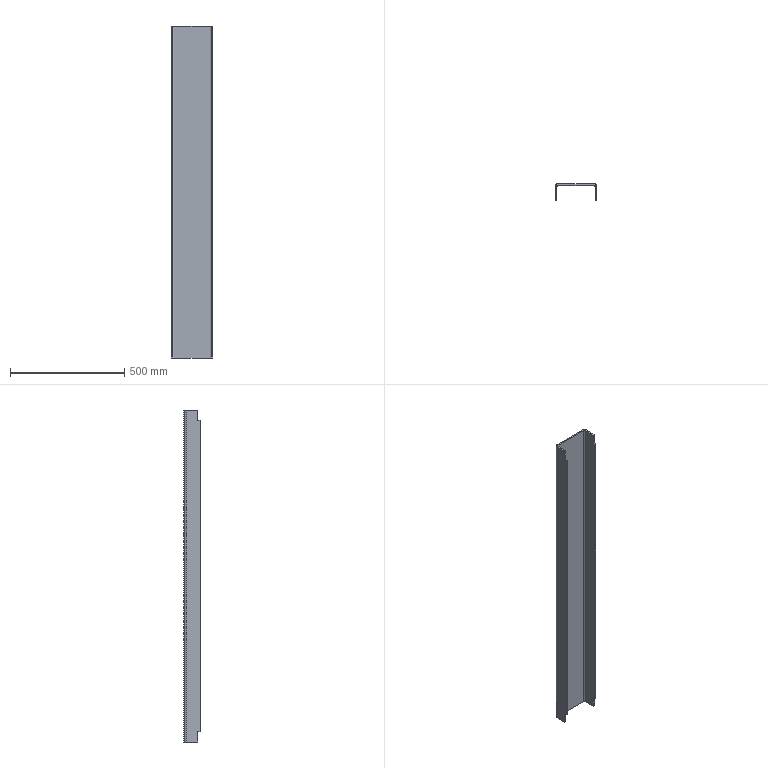Part | STEP file | VD-SYL0380DJ1006_1_1_2-1_VD-SYL | 1 solid | 30 faces | box 180 x 70 x 1450 mm | volume 2609055 mm3 | plane 26 | cylinder 4 | commonest cylinder face diameters 10 x2 22 x2
STEP:
#1=CARTESIAN_POINT('',(-90.,10.,725.));
#2=VERTEX_POINT('',#1);
#3=CARTESIAN_POINT('',(-90.,10.,680.));
#4=VERTEX_POINT('',#3);
#5=CARTESIAN_POINT('',(-90.,10.,725.));
#6=DIRECTION('',(0.,0.,-1.));
#7=VECTOR('',#6,1000.);
#8=LINE('',#5,#7);
#9=EDGE_CURVE('',#2,#4,#8,.T.);
#10=ORIENTED_EDGE('',*,*,#9,.F.);
#11=CARTESIAN_POINT('',(-90.,59.,725.));
#12=VERTEX_POINT('',#11);
#13=CARTESIAN_POINT('',(-90.,59.,725.));
#14=DIRECTION('',(0.,-1.,0.));
#15=VECTOR('',#14,1000.);
#16=LINE('',#13,#15);
#17=EDGE_CURVE('',#12,#2,#16,.T.);
#18=ORIENTED_EDGE('',*,*,#17,.F.);
#19=CARTESIAN_POINT('',(-90.,59.,-725.));
#20=VERTEX_POINT('',#19);
#21=CARTESIAN_POINT('',(-90.,59.,-725.));
#22=DIRECTION('',(0.,0.,1.));
#23=VECTOR('',#22,1000.);
#24=LINE('',#21,#23);
#25=EDGE_CURVE('',#20,#12,#24,.T.);
#26=ORIENTED_EDGE('',*,*,#25,.F.);
#27=CARTESIAN_POINT('',(-90.,10.,-725.));
#28=VERTEX_POINT('',#27);
#29=CARTESIAN_POINT('',(-90.,59.,-725.));
#30=DIRECTION('',(0.,-1.,0.));
#31=VECTOR('',#30,1000.);
#32=LINE('',#29,#31);
#33=EDGE_CURVE('',#20,#28,#32,.T.);
#34=ORIENTED_EDGE('',*,*,#33,.T.);
#35=CARTESIAN_POINT('',(-90.,10.,-680.));
#36=VERTEX_POINT('',#35);
#37=CARTESIAN_POINT('',(-90.,10.,-725.));
#38=DIRECTION('',(0.,0.,1.));
#39=VECTOR('',#38,1000.);
#40=LINE('',#37,#39);
#41=EDGE_CURVE('',#28,#36,#40,.T.);
#42=ORIENTED_EDGE('',*,*,#41,.T.);
#43=CARTESIAN_POINT('',(-90.,0.,-680.));
#44=VERTEX_POINT('',#43);
#45=CARTESIAN_POINT('',(-90.,0.,-680.));
#46=DIRECTION('',(0.,1.,0.));
#47=VECTOR('',#46,1000.);
#48=LINE('',#45,#47);
#49=EDGE_CURVE('',#44,#36,#48,.T.);
#50=ORIENTED_EDGE('',*,*,#49,.F.);
#51=CARTESIAN_POINT('',(-90.,0.,680.));
#52=VERTEX_POINT('',#51);
#53=CARTESIAN_POINT('',(-90.,0.,-680.));
#54=DIRECTION('',(0.,0.,1.));
#55=VECTOR('',#54,1000.);
#56=LINE('',#53,#55);
#57=EDGE_CURVE('',#44,#52,#56,.T.);
#58=ORIENTED_EDGE('',*,*,#57,.T.);
#59=CARTESIAN_POINT('',(-90.,0.,680.));
#60=DIRECTION('',(0.,1.,0.));
#61=VECTOR('',#60,1000.);
#62=LINE('',#59,#61);
#63=EDGE_CURVE('',#52,#4,#62,.T.);
#64=ORIENTED_EDGE('',*,*,#63,.T.);
#65=EDGE_LOOP('',(#10,#18,#26,#34,#42,#50,#58,#64));
#66=FACE_OUTER_BOUND('',#65,.T.);
#67=CARTESIAN_POINT('',(-90.,70.,-725.));
#68=DIRECTION('',(-1.,0.,0.));
#69=DIRECTION('',(0.,0.,1.));
#70=AXIS2_PLACEMENT_3D('',#67,#68,#69);
#71=PLANE('',#70);
#72=ADVANCED_FACE('',(#66),#71,.T.);
#73=ORIENTED_EDGE('',*,*,#25,.T.);
#74=CARTESIAN_POINT('',(-79.,70.,725.));
#75=VERTEX_POINT('',#74);
#76=CARTESIAN_POINT('',(-79.,59.,725.));
#77=DIRECTION('',(0.,0.,1.));
#78=DIRECTION('',(0.,1.,0.));
#79=AXIS2_PLACEMENT_3D('',#76,#77,#78);
#80=CIRCLE('',#79,11.);
#81=EDGE_CURVE('',#75,#12,#80,.T.);
#82=ORIENTED_EDGE('',*,*,#81,.F.);
#83=CARTESIAN_POINT('',(-79.,70.,-725.));
#84=VERTEX_POINT('',#83);
#85=CARTESIAN_POINT('',(-79.,70.,725.));
#86=DIRECTION('',(0.,0.,-1.));
#87=VECTOR('',#86,1000.);
#88=LINE('',#85,#87);
#89=EDGE_CURVE('',#75,#84,#88,.T.);
#90=ORIENTED_EDGE('',*,*,#89,.T.);
#91=CARTESIAN_POINT('',(-79.,59.,-725.));
#92=DIRECTION('',(0.,0.,-1.));
#93=DIRECTION('',(-1.,0.,0.));
#94=AXIS2_PLACEMENT_3D('',#91,#92,#93);
#95=CIRCLE('',#94,11.);
#96=EDGE_CURVE('',#20,#84,#95,.T.);
#97=ORIENTED_EDGE('',*,*,#96,.F.);
#98=EDGE_LOOP('',(#73,#82,#90,#97));
#99=FACE_OUTER_BOUND('',#98,.T.);
#100=CARTESIAN_POINT('',(-79.,59.,-725.));
#101=DIRECTION('',(0.,0.,-1.));
#102=DIRECTION('',(-1.,0.,0.));
#103=AXIS2_PLACEMENT_3D('',#100,#101,#102);
#104=CYLINDRICAL_SURFACE('',#103,11.);
#105=ADVANCED_FACE('',(#99),#104,.T.);
#106=CARTESIAN_POINT('',(79.,70.,-725.));
#107=VERTEX_POINT('',#106);
#108=CARTESIAN_POINT('',(79.,70.,-725.));
#109=DIRECTION('',(-1.,0.,0.));
#110=VECTOR('',#109,1000.);
#111=LINE('',#108,#110);
#112=EDGE_CURVE('',#107,#84,#111,.T.);
#113=ORIENTED_EDGE('',*,*,#112,.T.);
#114=ORIENTED_EDGE('',*,*,#89,.F.);
#115=CARTESIAN_POINT('',(79.,70.,725.));
#116=VERTEX_POINT('',#115);
#117=CARTESIAN_POINT('',(79.,70.,725.));
#118=DIRECTION('',(-1.,0.,0.));
#119=VECTOR('',#118,1000.);
#120=LINE('',#117,#119);
#121=EDGE_CURVE('',#116,#75,#120,.T.);
#122=ORIENTED_EDGE('',*,*,#121,.F.);
#123=CARTESIAN_POINT('',(79.,70.,-725.));
#124=DIRECTION('',(0.,0.,1.));
#125=VECTOR('',#124,1000.);
#126=LINE('',#123,#125);
#127=EDGE_CURVE('',#107,#116,#126,.T.);
#128=ORIENTED_EDGE('',*,*,#127,.F.);
#129=EDGE_LOOP('',(#113,#114,#122,#128));
#130=FACE_OUTER_BOUND('',#129,.T.);
#131=CARTESIAN_POINT('',(90.,70.,-725.));
#132=DIRECTION('',(0.,1.,0.));
#133=DIRECTION('',(1.,0.,0.));
#134=AXIS2_PLACEMENT_3D('',#131,#132,#133);
#135=PLANE('',#134);
#136=ADVANCED_FACE('',(#130),#135,.T.);
#137=ORIENTED_EDGE('',*,*,#127,.T.);
#138=CARTESIAN_POINT('',(90.,59.,725.));
#139=VERTEX_POINT('',#138);
#140=CARTESIAN_POINT('',(79.,59.,725.));
#141=DIRECTION('',(0.,0.,1.));
#142=DIRECTION('',(1.,0.,0.));
#143=AXIS2_PLACEMENT_3D('',#140,#141,#142);
#144=CIRCLE('',#143,11.);
#145=EDGE_CURVE('',#139,#116,#144,.T.);
#146=ORIENTED_EDGE('',*,*,#145,.F.);
#147=CARTESIAN_POINT('',(90.,59.,-725.));
#148=VERTEX_POINT('',#147);
#149=CARTESIAN_POINT('',(90.,59.,725.));
#150=DIRECTION('',(0.,0.,-1.));
#151=VECTOR('',#150,1000.);
#152=LINE('',#149,#151);
#153=EDGE_CURVE('',#139,#148,#152,.T.);
#154=ORIENTED_EDGE('',*,*,#153,.T.);
#155=CARTESIAN_POINT('',(79.,59.,-725.));
#156=DIRECTION('',(0.,0.,-1.));
#157=DIRECTION('',(0.,1.,0.));
#158=AXIS2_PLACEMENT_3D('',#155,#156,#157);
#159=CIRCLE('',#158,11.);
#160=EDGE_CURVE('',#107,#148,#159,.T.);
#161=ORIENTED_EDGE('',*,*,#160,.F.);
#162=EDGE_LOOP('',(#137,#146,#154,#161));
#163=FACE_OUTER_BOUND('',#162,.T.);
#164=CARTESIAN_POINT('',(79.,59.,-725.));
#165=DIRECTION('',(0.,0.,-1.));
#166=DIRECTION('',(-1.,0.,0.));
#167=AXIS2_PLACEMENT_3D('',#164,#165,#166);
#168=CYLINDRICAL_SURFACE('',#167,11.);
#169=ADVANCED_FACE('',(#163),#168,.T.);
#170=CARTESIAN_POINT('',(79.,64.,725.));
#171=VERTEX_POINT('',#170);
#172=CARTESIAN_POINT('',(-79.,64.,725.));
#173=VERTEX_POINT('',#172);
#174=CARTESIAN_POINT('',(79.,64.,725.));
#175=DIRECTION('',(-1.,0.,0.));
#176=VECTOR('',#175,1000.);
#177=LINE('',#174,#176);
#178=EDGE_CURVE('',#171,#173,#177,.T.);
#179=ORIENTED_EDGE('',*,*,#178,.T.);
#180=CARTESIAN_POINT('',(-79.,64.,-725.));
#181=VERTEX_POINT('',#180);
#182=CARTESIAN_POINT('',(-79.,64.,-725.));
#183=DIRECTION('',(0.,0.,1.));
#184=VECTOR('',#183,1000.);
#185=LINE('',#182,#184);
#186=EDGE_CURVE('',#181,#173,#185,.T.);
#187=ORIENTED_EDGE('',*,*,#186,.F.);
#188=CARTESIAN_POINT('',(79.,64.,-725.));
#189=VERTEX_POINT('',#188);
#190=CARTESIAN_POINT('',(79.,64.,-725.));
#191=DIRECTION('',(-1.,0.,0.));
#192=VECTOR('',#191,1000.);
#193=LINE('',#190,#192);
#194=EDGE_CURVE('',#189,#181,#193,.T.);
#195=ORIENTED_EDGE('',*,*,#194,.F.);
#196=CARTESIAN_POINT('',(79.,64.,725.));
#197=DIRECTION('',(0.,0.,-1.));
#198=VECTOR('',#197,1000.);
#199=LINE('',#196,#198);
#200=EDGE_CURVE('',#171,#189,#199,.T.);
#201=ORIENTED_EDGE('',*,*,#200,.F.);
#202=EDGE_LOOP('',(#179,#187,#195,#201));
#203=FACE_OUTER_BOUND('',#202,.T.);
#204=CARTESIAN_POINT('',(90.,64.,-725.));
#205=DIRECTION('',(0.,1.,0.));
#206=DIRECTION('',(1.,0.,0.));
#207=AXIS2_PLACEMENT_3D('',#204,#205,#206);
#208=PLANE('',#207);
#209=ADVANCED_FACE('',(#203),#208,.F.);
#210=CARTESIAN_POINT('',(84.,59.,-725.));
#211=VERTEX_POINT('',#210);
#212=CARTESIAN_POINT('',(84.,59.,725.));
#213=VERTEX_POINT('',#212);
#214=CARTESIAN_POINT('',(84.,59.,-725.));
#215=DIRECTION('',(0.,0.,1.));
#216=VECTOR('',#215,1000.);
#217=LINE('',#214,#216);
#218=EDGE_CURVE('',#211,#213,#217,.T.);
#219=ORIENTED_EDGE('',*,*,#218,.T.);
#220=CARTESIAN_POINT('',(79.,59.,725.));
#221=DIRECTION('',(0.,0.,-1.));
#222=DIRECTION('',(0.,1.,0.));
#223=AXIS2_PLACEMENT_3D('',#220,#221,#222);
#224=CIRCLE('',#223,5.);
#225=EDGE_CURVE('',#171,#213,#224,.T.);
#226=ORIENTED_EDGE('',*,*,#225,.F.);
#227=ORIENTED_EDGE('',*,*,#200,.T.);
#228=CARTESIAN_POINT('',(79.,59.,-725.));
#229=DIRECTION('',(0.,0.,1.));
#230=DIRECTION('',(1.,0.,0.));
#231=AXIS2_PLACEMENT_3D('',#228,#229,#230);
#232=CIRCLE('',#231,5.);
#233=EDGE_CURVE('',#211,#189,#232,.T.);
#234=ORIENTED_EDGE('',*,*,#233,.F.);
#235=EDGE_LOOP('',(#219,#226,#227,#234));
#236=FACE_OUTER_BOUND('',#235,.T.);
#237=CARTESIAN_POINT('',(79.,59.,-725.));
#238=DIRECTION('',(0.,0.,-1.));
#239=DIRECTION('',(-1.,0.,0.));
#240=AXIS2_PLACEMENT_3D('',#237,#238,#239);
#241=CYLINDRICAL_SURFACE('',#240,5.);
#242=ADVANCED_FACE('',(#236),#241,.F.);
#243=ORIENTED_EDGE('',*,*,#218,.F.);
#244=CARTESIAN_POINT('',(84.,10.,-725.));
#245=VERTEX_POINT('',#244);
#246=CARTESIAN_POINT('',(84.,10.,-725.));
#247=DIRECTION('',(0.,1.,0.));
#248=VECTOR('',#247,1000.);
#249=LINE('',#246,#248);
#250=EDGE_CURVE('',#245,#211,#249,.T.);
#251=ORIENTED_EDGE('',*,*,#250,.F.);
#252=CARTESIAN_POINT('',(84.,10.,-680.));
#253=VERTEX_POINT('',#252);
#254=CARTESIAN_POINT('',(84.,10.,-725.));
#255=DIRECTION('',(0.,0.,1.));
#256=VECTOR('',#255,1000.);
#257=LINE('',#254,#256);
#258=EDGE_CURVE('',#245,#253,#257,.T.);
#259=ORIENTED_EDGE('',*,*,#258,.T.);
#260=CARTESIAN_POINT('',(84.,0.,-680.));
#261=VERTEX_POINT('',#260);
#262=CARTESIAN_POINT('',(84.,0.,-680.));
#263=DIRECTION('',(0.,1.,0.));
#264=VECTOR('',#263,1000.);
#265=LINE('',#262,#264);
#266=EDGE_CURVE('',#261,#253,#265,.T.);
#267=ORIENTED_EDGE('',*,*,#266,.F.);
#268=CARTESIAN_POINT('',(84.,0.,680.));
#269=VERTEX_POINT('',#268);
#270=CARTESIAN_POINT('',(84.,0.,-680.));
#271=DIRECTION('',(0.,0.,1.));
#272=VECTOR('',#271,1000.);
#273=LINE('',#270,#272);
#274=EDGE_CURVE('',#261,#269,#273,.T.);
#275=ORIENTED_EDGE('',*,*,#274,.T.);
#276=CARTESIAN_POINT('',(84.,10.,680.));
#277=VERTEX_POINT('',#276);
#278=CARTESIAN_POINT('',(84.,0.,680.));
#279=DIRECTION('',(0.,1.,0.));
#280=VECTOR('',#279,1000.);
#281=LINE('',#278,#280);
#282=EDGE_CURVE('',#269,#277,#281,.T.);
#283=ORIENTED_EDGE('',*,*,#282,.T.);
#284=CARTESIAN_POINT('',(84.,10.,725.));
#285=VERTEX_POINT('',#284);
#286=CARTESIAN_POINT('',(84.,10.,725.));
#287=DIRECTION('',(0.,0.,-1.));
#288=VECTOR('',#287,1000.);
#289=LINE('',#286,#288);
#290=EDGE_CURVE('',#285,#277,#289,.T.);
#291=ORIENTED_EDGE('',*,*,#290,.F.);
#292=CARTESIAN_POINT('',(84.,10.,725.));
#293=DIRECTION('',(0.,1.,0.));
#294=VECTOR('',#293,1000.);
#295=LINE('',#292,#294);
#296=EDGE_CURVE('',#285,#213,#295,.T.);
#297=ORIENTED_EDGE('',*,*,#296,.T.);
#298=EDGE_LOOP('',(#243,#251,#259,#267,#275,#283,#291,#297));
#299=FACE_OUTER_BOUND('',#298,.T.);
#300=CARTESIAN_POINT('',(84.,0.,-725.));
#301=DIRECTION('',(1.,0.,0.));
#302=DIRECTION('',(0.,1.,0.));
#303=AXIS2_PLACEMENT_3D('',#300,#301,#302);
#304=PLANE('',#303);
#305=ADVANCED_FACE('',(#299),#304,.F.);
#306=ORIENTED_EDGE('',*,*,#290,.T.);
#307=CARTESIAN_POINT('',(90.,10.,680.));
#308=VERTEX_POINT('',#307);
#309=CARTESIAN_POINT('',(90.,10.,680.));
#310=DIRECTION('',(-1.,0.,0.));
#311=VECTOR('',#310,1000.);
#312=LINE('',#309,#311);
#313=EDGE_CURVE('',#308,#277,#312,.T.);
#314=ORIENTED_EDGE('',*,*,#313,.F.);
#315=CARTESIAN_POINT('',(90.,10.,725.));
#316=VERTEX_POINT('',#315);
#317=CARTESIAN_POINT('',(90.,10.,725.));
#318=DIRECTION('',(0.,0.,-1.));
#319=VECTOR('',#318,1000.);
#320=LINE('',#317,#319);
#321=EDGE_CURVE('',#316,#308,#320,.T.);
#322=ORIENTED_EDGE('',*,*,#321,.F.);
#323=CARTESIAN_POINT('',(90.,10.,725.));
#324=DIRECTION('',(-1.,0.,0.));
#325=VECTOR('',#324,1000.);
#326=LINE('',#323,#325);
#327=EDGE_CURVE('',#316,#285,#326,.T.);
#328=ORIENTED_EDGE('',*,*,#327,.T.);
#329=EDGE_LOOP('',(#306,#314,#322,#328));
#330=FACE_OUTER_BOUND('',#329,.T.);
#331=CARTESIAN_POINT('',(90.,10.,702.5));
#332=DIRECTION('',(0.,-1.,0.));
#333=DIRECTION('',(0.,0.,-1.));
#334=AXIS2_PLACEMENT_3D('',#331,#332,#333);
#335=PLANE('',#334);
#336=ADVANCED_FACE('',(#330),#335,.T.);
#337=ORIENTED_EDGE('',*,*,#282,.F.);
#338=CARTESIAN_POINT('',(90.,0.,680.));
#339=VERTEX_POINT('',#338);
#340=CARTESIAN_POINT('',(90.,0.,680.));
#341=DIRECTION('',(-1.,0.,0.));
#342=VECTOR('',#341,1000.);
#343=LINE('',#340,#342);
#344=EDGE_CURVE('',#339,#269,#343,.T.);
#345=ORIENTED_EDGE('',*,*,#344,.F.);
#346=CARTESIAN_POINT('',(90.,0.,680.));
#347=DIRECTION('',(0.,1.,0.));
#348=VECTOR('',#347,1000.);
#349=LINE('',#346,#348);
#350=EDGE_CURVE('',#339,#308,#349,.T.);
#351=ORIENTED_EDGE('',*,*,#350,.T.);
#352=ORIENTED_EDGE('',*,*,#313,.T.);
#353=EDGE_LOOP('',(#337,#345,#351,#352));
#354=FACE_OUTER_BOUND('',#353,.T.);
#355=CARTESIAN_POINT('',(90.,5.,680.));
#356=DIRECTION('',(0.,0.,-1.));
#357=DIRECTION('',(0.,-1.,0.));
#358=AXIS2_PLACEMENT_3D('',#355,#356,#357);
#359=PLANE('',#358);
#360=ADVANCED_FACE('',(#354),#359,.F.);
#361=ORIENTED_EDGE('',*,*,#274,.F.);
#362=CARTESIAN_POINT('',(90.,0.,-680.));
#363=VERTEX_POINT('',#362);
#364=CARTESIAN_POINT('',(90.,0.,-680.));
#365=DIRECTION('',(-1.,0.,0.));
#366=VECTOR('',#365,1000.);
#367=LINE('',#364,#366);
#368=EDGE_CURVE('',#363,#261,#367,.T.);
#369=ORIENTED_EDGE('',*,*,#368,.F.);
#370=CARTESIAN_POINT('',(90.,0.,-680.));
#371=DIRECTION('',(0.,0.,1.));
#372=VECTOR('',#371,1000.);
#373=LINE('',#370,#372);
#374=EDGE_CURVE('',#363,#339,#373,.T.);
#375=ORIENTED_EDGE('',*,*,#374,.T.);
#376=ORIENTED_EDGE('',*,*,#344,.T.);
#377=EDGE_LOOP('',(#361,#369,#375,#376));
#378=FACE_OUTER_BOUND('',#377,.T.);
#379=CARTESIAN_POINT('',(90.,0.,0.));
#380=DIRECTION('',(0.,1.,0.));
#381=DIRECTION('',(1.,0.,0.));
#382=AXIS2_PLACEMENT_3D('',#379,#380,#381);
#383=PLANE('',#382);
#384=ADVANCED_FACE('',(#378),#383,.F.);
#385=ORIENTED_EDGE('',*,*,#266,.T.);
#386=CARTESIAN_POINT('',(90.,10.,-680.));
#387=VERTEX_POINT('',#386);
#388=CARTESIAN_POINT('',(90.,10.,-680.));
#389=DIRECTION('',(-1.,0.,0.));
#390=VECTOR('',#389,1000.);
#391=LINE('',#388,#390);
#392=EDGE_CURVE('',#387,#253,#391,.T.);
#393=ORIENTED_EDGE('',*,*,#392,.F.);
#394=CARTESIAN_POINT('',(90.,0.,-680.));
#395=DIRECTION('',(0.,1.,0.));
#396=VECTOR('',#395,1000.);
#397=LINE('',#394,#396);
#398=EDGE_CURVE('',#363,#387,#397,.T.);
#399=ORIENTED_EDGE('',*,*,#398,.F.);
#400=ORIENTED_EDGE('',*,*,#368,.T.);
#401=EDGE_LOOP('',(#385,#393,#399,#400));
#402=FACE_OUTER_BOUND('',#401,.T.);
#403=CARTESIAN_POINT('',(90.,5.,-680.));
#404=DIRECTION('',(0.,0.,-1.));
#405=DIRECTION('',(0.,-1.,0.));
#406=AXIS2_PLACEMENT_3D('',#403,#404,#405);
#407=PLANE('',#406);
#408=ADVANCED_FACE('',(#402),#407,.T.);
#409=ORIENTED_EDGE('',*,*,#258,.F.);
#410=CARTESIAN_POINT('',(90.,10.,-725.));
#411=VERTEX_POINT('',#410);
#412=CARTESIAN_POINT('',(90.,10.,-725.));
#413=DIRECTION('',(-1.,0.,0.));
#414=VECTOR('',#413,1000.);
#415=LINE('',#412,#414);
#416=EDGE_CURVE('',#411,#245,#415,.T.);
#417=ORIENTED_EDGE('',*,*,#416,.F.);
#418=CARTESIAN_POINT('',(90.,10.,-725.));
#419=DIRECTION('',(0.,0.,1.));
#420=VECTOR('',#419,1000.);
#421=LINE('',#418,#420);
#422=EDGE_CURVE('',#411,#387,#421,.T.);
#423=ORIENTED_EDGE('',*,*,#422,.T.);
#424=ORIENTED_EDGE('',*,*,#392,.T.);
#425=EDGE_LOOP('',(#409,#417,#423,#424));
#426=FACE_OUTER_BOUND('',#425,.T.);
#427=CARTESIAN_POINT('',(90.,10.,-702.5));
#428=DIRECTION('',(0.,1.,0.));
#429=DIRECTION('',(1.,0.,0.));
#430=AXIS2_PLACEMENT_3D('',#427,#428,#429);
#431=PLANE('',#430);
#432=ADVANCED_FACE('',(#426),#431,.F.);
#433=ORIENTED_EDGE('',*,*,#250,.T.);
#434=CARTESIAN_POINT('',(90.,59.,-725.));
#435=DIRECTION('',(-1.,0.,0.));
#436=VECTOR('',#435,1000.);
#437=LINE('',#434,#436);
#438=EDGE_CURVE('',#148,#211,#437,.T.);
#439=ORIENTED_EDGE('',*,*,#438,.F.);
#440=CARTESIAN_POINT('',(90.,10.,-725.));
#441=DIRECTION('',(0.,1.,0.));
#442=VECTOR('',#441,1000.);
#443=LINE('',#440,#442);
#444=EDGE_CURVE('',#411,#148,#443,.T.);
#445=ORIENTED_EDGE('',*,*,#444,.F.);
#446=ORIENTED_EDGE('',*,*,#416,.T.);
#447=EDGE_LOOP('',(#433,#439,#445,#446));
#448=FACE_OUTER_BOUND('',#447,.T.);
#449=CARTESIAN_POINT('',(90.,29.5,-725.));
#450=DIRECTION('',(0.,0.,-1.));
#451=DIRECTION('',(0.,-1.,0.));
#452=AXIS2_PLACEMENT_3D('',#449,#450,#451);
#453=PLANE('',#452);
#454=ADVANCED_FACE('',(#448),#453,.T.);
#455=ORIENTED_EDGE('',*,*,#233,.T.);
#456=CARTESIAN_POINT('',(79.,70.,-725.));
#457=DIRECTION('',(0.,-1.,0.));
#458=VECTOR('',#457,1000.);
#459=LINE('',#456,#458);
#460=EDGE_CURVE('',#107,#189,#459,.T.);
#461=ORIENTED_EDGE('',*,*,#460,.F.);
#462=ORIENTED_EDGE('',*,*,#160,.T.);
#463=ORIENTED_EDGE('',*,*,#438,.T.);
#464=EDGE_LOOP('',(#455,#461,#462,#463));
#465=FACE_OUTER_BOUND('',#464,.T.);
#466=CARTESIAN_POINT('',(79.,59.,-725.));
#467=DIRECTION('',(0.,0.,1.));
#468=DIRECTION('',(1.,0.,0.));
#469=AXIS2_PLACEMENT_3D('',#466,#467,#468);
#470=PLANE('',#469);
#471=ADVANCED_FACE('',(#465),#470,.F.);
#472=ORIENTED_EDGE('',*,*,#194,.T.);
#473=CARTESIAN_POINT('',(-79.,70.,-725.));
#474=DIRECTION('',(0.,-1.,0.));
#475=VECTOR('',#474,1000.);
#476=LINE('',#473,#475);
#477=EDGE_CURVE('',#84,#181,#476,.T.);
#478=ORIENTED_EDGE('',*,*,#477,.F.);
#479=ORIENTED_EDGE('',*,*,#112,.F.);
#480=ORIENTED_EDGE('',*,*,#460,.T.);
#481=EDGE_LOOP('',(#472,#478,#479,#480));
#482=FACE_OUTER_BOUND('',#481,.T.);
#483=CARTESIAN_POINT('',(0.,70.,-725.));
#484=DIRECTION('',(0.,0.,-1.));
#485=DIRECTION('',(0.,-1.,0.));
#486=AXIS2_PLACEMENT_3D('',#483,#484,#485);
#487=PLANE('',#486);
#488=ADVANCED_FACE('',(#482),#487,.T.);
#489=CARTESIAN_POINT('',(-84.,59.,-725.));
#490=VERTEX_POINT('',#489);
#491=CARTESIAN_POINT('',(-79.,59.,-725.));
#492=DIRECTION('',(0.,0.,1.));
#493=DIRECTION('',(0.,1.,0.));
#494=AXIS2_PLACEMENT_3D('',#491,#492,#493);
#495=CIRCLE('',#494,5.);
#496=EDGE_CURVE('',#181,#490,#495,.T.);
#497=ORIENTED_EDGE('',*,*,#496,.T.);
#498=CARTESIAN_POINT('',(-90.,59.,-725.));
#499=DIRECTION('',(1.,0.,0.));
#500=VECTOR('',#499,1000.);
#501=LINE('',#498,#500);
#502=EDGE_CURVE('',#20,#490,#501,.T.);
#503=ORIENTED_EDGE('',*,*,#502,.F.);
#504=ORIENTED_EDGE('',*,*,#96,.T.);
#505=ORIENTED_EDGE('',*,*,#477,.T.);
#506=EDGE_LOOP('',(#497,#503,#504,#505));
#507=FACE_OUTER_BOUND('',#506,.T.);
#508=CARTESIAN_POINT('',(-79.,59.,-725.));
#509=DIRECTION('',(0.,0.,1.));
#510=DIRECTION('',(1.,0.,0.));
#511=AXIS2_PLACEMENT_3D('',#508,#509,#510);
#512=PLANE('',#511);
#513=ADVANCED_FACE('',(#507),#512,.F.);
#514=ORIENTED_EDGE('',*,*,#186,.T.);
#515=CARTESIAN_POINT('',(-84.,59.,725.));
#516=VERTEX_POINT('',#515);
#517=CARTESIAN_POINT('',(-79.,59.,725.));
#518=DIRECTION('',(0.,0.,-1.));
#519=DIRECTION('',(-1.,0.,0.));
#520=AXIS2_PLACEMENT_3D('',#517,#518,#519);
#521=CIRCLE('',#520,5.);
#522=EDGE_CURVE('',#516,#173,#521,.T.);
#523=ORIENTED_EDGE('',*,*,#522,.F.);
#524=CARTESIAN_POINT('',(-84.,59.,725.));
#525=DIRECTION('',(0.,0.,-1.));
#526=VECTOR('',#525,1000.);
#527=LINE('',#524,#526);
#528=EDGE_CURVE('',#516,#490,#527,.T.);
#529=ORIENTED_EDGE('',*,*,#528,.T.);
#530=ORIENTED_EDGE('',*,*,#496,.F.);
#531=EDGE_LOOP('',(#514,#523,#529,#530));
#532=FACE_OUTER_BOUND('',#531,.T.);
#533=CARTESIAN_POINT('',(-79.,59.,-725.));
#534=DIRECTION('',(0.,0.,-1.));
#535=DIRECTION('',(-1.,0.,0.));
#536=AXIS2_PLACEMENT_3D('',#533,#534,#535);
#537=CYLINDRICAL_SURFACE('',#536,5.);
#538=ADVANCED_FACE('',(#532),#537,.F.);
#539=CARTESIAN_POINT('',(-84.,0.,-680.));
#540=VERTEX_POINT('',#539);
#541=CARTESIAN_POINT('',(-84.,0.,680.));
#542=VERTEX_POINT('',#541);
#543=CARTESIAN_POINT('',(-84.,0.,-680.));
#544=DIRECTION('',(0.,0.,1.));
#545=VECTOR('',#544,1000.);
#546=LINE('',#543,#545);
#547=EDGE_CURVE('',#540,#542,#546,.T.);
#548=ORIENTED_EDGE('',*,*,#547,.F.);
#549=CARTESIAN_POINT('',(-84.,10.,-680.));
#550=VERTEX_POINT('',#549);
#551=CARTESIAN_POINT('',(-84.,0.,-680.));
#552=DIRECTION('',(0.,1.,0.));
#553=VECTOR('',#552,1000.);
#554=LINE('',#551,#553);
#555=EDGE_CURVE('',#540,#550,#554,.T.);
#556=ORIENTED_EDGE('',*,*,#555,.T.);
#557=CARTESIAN_POINT('',(-84.,10.,-725.));
#558=VERTEX_POINT('',#557);
#559=CARTESIAN_POINT('',(-84.,10.,-725.));
#560=DIRECTION('',(0.,0.,1.));
#561=VECTOR('',#560,1000.);
#562=LINE('',#559,#561);
#563=EDGE_CURVE('',#558,#550,#562,.T.);
#564=ORIENTED_EDGE('',*,*,#563,.F.);
#565=CARTESIAN_POINT('',(-84.,59.,-725.));
#566=DIRECTION('',(0.,-1.,0.));
#567=VECTOR('',#566,1000.);
#568=LINE('',#565,#567);
#569=EDGE_CURVE('',#490,#558,#568,.T.);
#570=ORIENTED_EDGE('',*,*,#569,.F.);
#571=ORIENTED_EDGE('',*,*,#528,.F.);
#572=CARTESIAN_POINT('',(-84.,10.,725.));
#573=VERTEX_POINT('',#572);
#574=CARTESIAN_POINT('',(-84.,59.,725.));
#575=DIRECTION('',(0.,-1.,0.));
#576=VECTOR('',#575,1000.);
#577=LINE('',#574,#576);
#578=EDGE_CURVE('',#516,#573,#577,.T.);
#579=ORIENTED_EDGE('',*,*,#578,.T.);
#580=CARTESIAN_POINT('',(-84.,10.,680.));
#581=VERTEX_POINT('',#580);
#582=CARTESIAN_POINT('',(-84.,10.,725.));
#583=DIRECTION('',(0.,0.,-1.));
#584=VECTOR('',#583,1000.);
#585=LINE('',#582,#584);
#586=EDGE_CURVE('',#573,#581,#585,.T.);
#587=ORIENTED_EDGE('',*,*,#586,.T.);
#588=CARTESIAN_POINT('',(-84.,0.,680.));
#589=DIRECTION('',(0.,1.,0.));
#590=VECTOR('',#589,1000.);
#591=LINE('',#588,#590);
#592=EDGE_CURVE('',#542,#581,#591,.T.);
#593=ORIENTED_EDGE('',*,*,#592,.F.);
#594=EDGE_LOOP('',(#548,#556,#564,#570,#571,#579,#587,#593));
#595=FACE_OUTER_BOUND('',#594,.T.);
#596=CARTESIAN_POINT('',(-84.,70.,-725.));
#597=DIRECTION('',(-1.,0.,0.));
#598=DIRECTION('',(0.,0.,1.));
#599=AXIS2_PLACEMENT_3D('',#596,#597,#598);
#600=PLANE('',#599);
#601=ADVANCED_FACE('',(#595),#600,.F.);
#602=CARTESIAN_POINT('',(-90.,10.,-725.));
#603=DIRECTION('',(1.,0.,0.));
#604=VECTOR('',#603,1000.);
#605=LINE('',#602,#604);
#606=EDGE_CURVE('',#28,#558,#605,.T.);
#607=ORIENTED_EDGE('',*,*,#606,.F.);
#608=ORIENTED_EDGE('',*,*,#33,.F.);
#609=ORIENTED_EDGE('',*,*,#502,.T.);
#610=ORIENTED_EDGE('',*,*,#569,.T.);
#611=EDGE_LOOP('',(#607,#608,#609,#610));
#612=FACE_OUTER_BOUND('',#611,.T.);
#613=CARTESIAN_POINT('',(-90.,29.5,-725.));
#614=DIRECTION('',(0.,0.,1.));
#615=DIRECTION('',(1.,0.,0.));
#616=AXIS2_PLACEMENT_3D('',#613,#614,#615);
#617=PLANE('',#616);
#618=ADVANCED_FACE('',(#612),#617,.F.);
#619=ORIENTED_EDGE('',*,*,#563,.T.);
#620=CARTESIAN_POINT('',(-90.,10.,-680.));
#621=DIRECTION('',(1.,0.,0.));
#622=VECTOR('',#621,1000.);
#623=LINE('',#620,#622);
#624=EDGE_CURVE('',#36,#550,#623,.T.);
#625=ORIENTED_EDGE('',*,*,#624,.F.);
#626=ORIENTED_EDGE('',*,*,#41,.F.);
#627=ORIENTED_EDGE('',*,*,#606,.T.);
#628=EDGE_LOOP('',(#619,#625,#626,#627));
#629=FACE_OUTER_BOUND('',#628,.T.);
#630=CARTESIAN_POINT('',(-90.,10.,-702.5));
#631=DIRECTION('',(0.,1.,0.));
#632=DIRECTION('',(1.,0.,0.));
#633=AXIS2_PLACEMENT_3D('',#630,#631,#632);
#634=PLANE('',#633);
#635=ADVANCED_FACE('',(#629),#634,.F.);
#636=ORIENTED_EDGE('',*,*,#555,.F.);
#637=CARTESIAN_POINT('',(-90.,0.,-680.));
#638=DIRECTION('',(1.,0.,0.));
#639=VECTOR('',#638,1000.);
#640=LINE('',#637,#639);
#641=EDGE_CURVE('',#44,#540,#640,.T.);
#642=ORIENTED_EDGE('',*,*,#641,.F.);
#643=ORIENTED_EDGE('',*,*,#49,.T.);
#644=ORIENTED_EDGE('',*,*,#624,.T.);
#645=EDGE_LOOP('',(#636,#642,#643,#644));
#646=FACE_OUTER_BOUND('',#645,.T.);
#647=CARTESIAN_POINT('',(-90.,5.,-680.));
#648=DIRECTION('',(0.,0.,1.));
#649=DIRECTION('',(1.,0.,0.));
#650=AXIS2_PLACEMENT_3D('',#647,#648,#649);
#651=PLANE('',#650);
#652=ADVANCED_FACE('',(#646),#651,.F.);
#653=ORIENTED_EDGE('',*,*,#547,.T.);
#654=CARTESIAN_POINT('',(-90.,0.,680.));
#655=DIRECTION('',(1.,0.,0.));
#656=VECTOR('',#655,1000.);
#657=LINE('',#654,#656);
#658=EDGE_CURVE('',#52,#542,#657,.T.);
#659=ORIENTED_EDGE('',*,*,#658,.F.);
#660=ORIENTED_EDGE('',*,*,#57,.F.);
#661=ORIENTED_EDGE('',*,*,#641,.T.);
#662=EDGE_LOOP('',(#653,#659,#660,#661));
#663=FACE_OUTER_BOUND('',#662,.T.);
#664=CARTESIAN_POINT('',(-90.,0.,0.));
#665=DIRECTION('',(0.,1.,0.));
#666=DIRECTION('',(1.,0.,0.));
#667=AXIS2_PLACEMENT_3D('',#664,#665,#666);
#668=PLANE('',#667);
#669=ADVANCED_FACE('',(#663),#668,.F.);
#670=ORIENTED_EDGE('',*,*,#592,.T.);
#671=CARTESIAN_POINT('',(-90.,10.,680.));
#672=DIRECTION('',(1.,0.,0.));
#673=VECTOR('',#672,1000.);
#674=LINE('',#671,#673);
#675=EDGE_CURVE('',#4,#581,#674,.T.);
#676=ORIENTED_EDGE('',*,*,#675,.F.);
#677=ORIENTED_EDGE('',*,*,#63,.F.);
#678=ORIENTED_EDGE('',*,*,#658,.T.);
#679=EDGE_LOOP('',(#670,#676,#677,#678));
#680=FACE_OUTER_BOUND('',#679,.T.);
#681=CARTESIAN_POINT('',(-90.,5.,680.));
#682=DIRECTION('',(0.,0.,1.));
#683=DIRECTION('',(1.,0.,0.));
#684=AXIS2_PLACEMENT_3D('',#681,#682,#683);
#685=PLANE('',#684);
#686=ADVANCED_FACE('',(#680),#685,.T.);
#687=ORIENTED_EDGE('',*,*,#586,.F.);
#688=CARTESIAN_POINT('',(-90.,10.,725.));
#689=DIRECTION('',(1.,0.,0.));
#690=VECTOR('',#689,1000.);
#691=LINE('',#688,#690);
#692=EDGE_CURVE('',#2,#573,#691,.T.);
#693=ORIENTED_EDGE('',*,*,#692,.F.);
#694=ORIENTED_EDGE('',*,*,#9,.T.);
#695=ORIENTED_EDGE('',*,*,#675,.T.);
#696=EDGE_LOOP('',(#687,#693,#694,#695));
#697=FACE_OUTER_BOUND('',#696,.T.);
#698=CARTESIAN_POINT('',(-90.,10.,702.5));
#699=DIRECTION('',(0.,-1.,0.));
#700=DIRECTION('',(0.,0.,-1.));
#701=AXIS2_PLACEMENT_3D('',#698,#699,#700);
#702=PLANE('',#701);
#703=ADVANCED_FACE('',(#697),#702,.T.);
#704=ORIENTED_EDGE('',*,*,#578,.F.);
#705=CARTESIAN_POINT('',(-90.,59.,725.));
#706=DIRECTION('',(1.,0.,0.));
#707=VECTOR('',#706,1000.);
#708=LINE('',#705,#707);
#709=EDGE_CURVE('',#12,#516,#708,.T.);
#710=ORIENTED_EDGE('',*,*,#709,.F.);
#711=ORIENTED_EDGE('',*,*,#17,.T.);
#712=ORIENTED_EDGE('',*,*,#692,.T.);
#713=EDGE_LOOP('',(#704,#710,#711,#712));
#714=FACE_OUTER_BOUND('',#713,.T.);
#715=CARTESIAN_POINT('',(-90.,29.5,725.));
#716=DIRECTION('',(0.,0.,1.));
#717=DIRECTION('',(1.,0.,0.));
#718=AXIS2_PLACEMENT_3D('',#715,#716,#717);
#719=PLANE('',#718);
#720=ADVANCED_FACE('',(#714),#719,.T.);
#721=ORIENTED_EDGE('',*,*,#522,.T.);
#722=CARTESIAN_POINT('',(-79.,70.,725.));
#723=DIRECTION('',(0.,-1.,0.));
#724=VECTOR('',#723,1000.);
#725=LINE('',#722,#724);
#726=EDGE_CURVE('',#75,#173,#725,.T.);
#727=ORIENTED_EDGE('',*,*,#726,.F.);
#728=ORIENTED_EDGE('',*,*,#81,.T.);
#729=ORIENTED_EDGE('',*,*,#709,.T.);
#730=EDGE_LOOP('',(#721,#727,#728,#729));
#731=FACE_OUTER_BOUND('',#730,.T.);
#732=CARTESIAN_POINT('',(-79.,59.,725.));
#733=DIRECTION('',(0.,0.,1.));
#734=DIRECTION('',(1.,0.,0.));
#735=AXIS2_PLACEMENT_3D('',#732,#733,#734);
#736=PLANE('',#735);
#737=ADVANCED_FACE('',(#731),#736,.T.);
#738=ORIENTED_EDGE('',*,*,#178,.F.);
#739=CARTESIAN_POINT('',(79.,70.,725.));
#740=DIRECTION('',(0.,-1.,0.));
#741=VECTOR('',#740,1000.);
#742=LINE('',#739,#741);
#743=EDGE_CURVE('',#116,#171,#742,.T.);
#744=ORIENTED_EDGE('',*,*,#743,.F.);
#745=ORIENTED_EDGE('',*,*,#121,.T.);
#746=ORIENTED_EDGE('',*,*,#726,.T.);
#747=EDGE_LOOP('',(#738,#744,#745,#746));
#748=FACE_OUTER_BOUND('',#747,.T.);
#749=CARTESIAN_POINT('',(0.,70.,725.));
#750=DIRECTION('',(0.,0.,1.));
#751=DIRECTION('',(1.,0.,0.));
#752=AXIS2_PLACEMENT_3D('',#749,#750,#751);
#753=PLANE('',#752);
#754=ADVANCED_FACE('',(#748),#753,.T.);
#755=ORIENTED_EDGE('',*,*,#225,.T.);
#756=CARTESIAN_POINT('',(90.,59.,725.));
#757=DIRECTION('',(-1.,0.,0.));
#758=VECTOR('',#757,1000.);
#759=LINE('',#756,#758);
#760=EDGE_CURVE('',#139,#213,#759,.T.);
#761=ORIENTED_EDGE('',*,*,#760,.F.);
#762=ORIENTED_EDGE('',*,*,#145,.T.);
#763=ORIENTED_EDGE('',*,*,#743,.T.);
#764=EDGE_LOOP('',(#755,#761,#762,#763));
#765=FACE_OUTER_BOUND('',#764,.T.);
#766=CARTESIAN_POINT('',(79.,59.,725.));
#767=DIRECTION('',(0.,0.,1.));
#768=DIRECTION('',(1.,0.,0.));
#769=AXIS2_PLACEMENT_3D('',#766,#767,#768);
#770=PLANE('',#769);
#771=ADVANCED_FACE('',(#765),#770,.T.);
#772=ORIENTED_EDGE('',*,*,#296,.F.);
#773=ORIENTED_EDGE('',*,*,#327,.F.);
#774=CARTESIAN_POINT('',(90.,10.,725.));
#775=DIRECTION('',(0.,1.,0.));
#776=VECTOR('',#775,1000.);
#777=LINE('',#774,#776);
#778=EDGE_CURVE('',#316,#139,#777,.T.);
#779=ORIENTED_EDGE('',*,*,#778,.T.);
#780=ORIENTED_EDGE('',*,*,#760,.T.);
#781=EDGE_LOOP('',(#772,#773,#779,#780));
#782=FACE_OUTER_BOUND('',#781,.T.);
#783=CARTESIAN_POINT('',(90.,29.5,725.));
#784=DIRECTION('',(0.,0.,-1.));
#785=DIRECTION('',(0.,-1.,0.));
#786=AXIS2_PLACEMENT_3D('',#783,#784,#785);
#787=PLANE('',#786);
#788=ADVANCED_FACE('',(#782),#787,.F.);
#789=ORIENTED_EDGE('',*,*,#321,.T.);
#790=ORIENTED_EDGE('',*,*,#350,.F.);
#791=ORIENTED_EDGE('',*,*,#374,.F.);
#792=ORIENTED_EDGE('',*,*,#398,.T.);
#793=ORIENTED_EDGE('',*,*,#422,.F.);
#794=ORIENTED_EDGE('',*,*,#444,.T.);
#795=ORIENTED_EDGE('',*,*,#153,.F.);
#796=ORIENTED_EDGE('',*,*,#778,.F.);
#797=EDGE_LOOP('',(#789,#790,#791,#792,#793,#794,#795,#796));
#798=FACE_OUTER_BOUND('',#797,.T.);
#799=CARTESIAN_POINT('',(90.,0.,-725.));
#800=DIRECTION('',(1.,0.,0.));
#801=DIRECTION('',(0.,1.,0.));
#802=AXIS2_PLACEMENT_3D('',#799,#800,#801);
#803=PLANE('',#802);
#804=ADVANCED_FACE('',(#798),#803,.T.);
#805=CLOSED_SHELL('',(#72,#105,#136,#169,#209,#242,#305,#336,#360,#384,#408,#432,#454,#471,#488,#513,#538,#601,#618,#635,#652,#669,#686,#703,#720,#737,#754,#771,#788,#804));
#806=MANIFOLD_SOLID_BREP('',#805);
#807=CARTESIAN_POINT('',(0.,0.,0.));
#808=DIRECTION('',(0.,0.,1.));
#809=DIRECTION('',(1.,0.,0.));
#810=AXIS2_PLACEMENT_3D('',#807,#808,#809);
#811=(LENGTH_UNIT()NAMED_UNIT(*)SI_UNIT(.MILLI.,.METRE.));
#812=UNCERTAINTY_MEASURE_WITH_UNIT(LENGTH_MEASURE(0.00001),#811,'','');
#813=(NAMED_UNIT(*)PLANE_ANGLE_UNIT()SI_UNIT($,.RADIAN.));
#814=(NAMED_UNIT(*)SI_UNIT($,.STERADIAN.)SOLID_ANGLE_UNIT());
#815=(GEOMETRIC_REPRESENTATION_CONTEXT(3)GLOBAL_UNCERTAINTY_ASSIGNED_CONTEXT((#812))GLOBAL_UNIT_ASSIGNED_CONTEXT((#811,#813,#814))REPRESENTATION_CONTEXT('',''));
#816=ADVANCED_BREP_SHAPE_REPRESENTATION('',(#806,#810),#815);